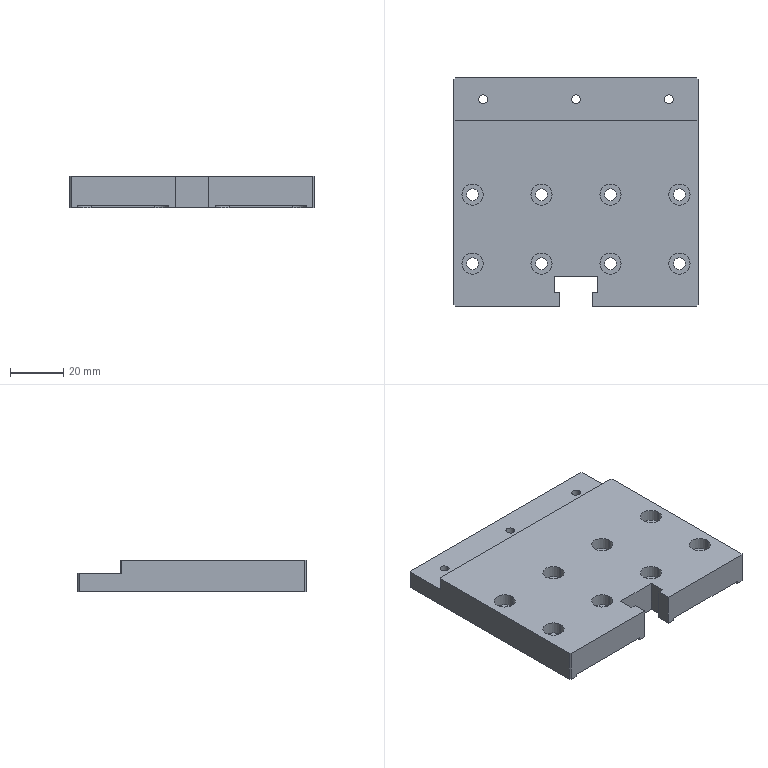Part | STEP file | 2028 Slider block connecting plate 1 | 1 solid | 80 faces | box 92 x 86 x 12 mm | volume 78738 mm3 | cylinder 42 | plane 38 | commonest cylinder face diameters 4.5 x16 8 x16 3.3 x6 10 x4